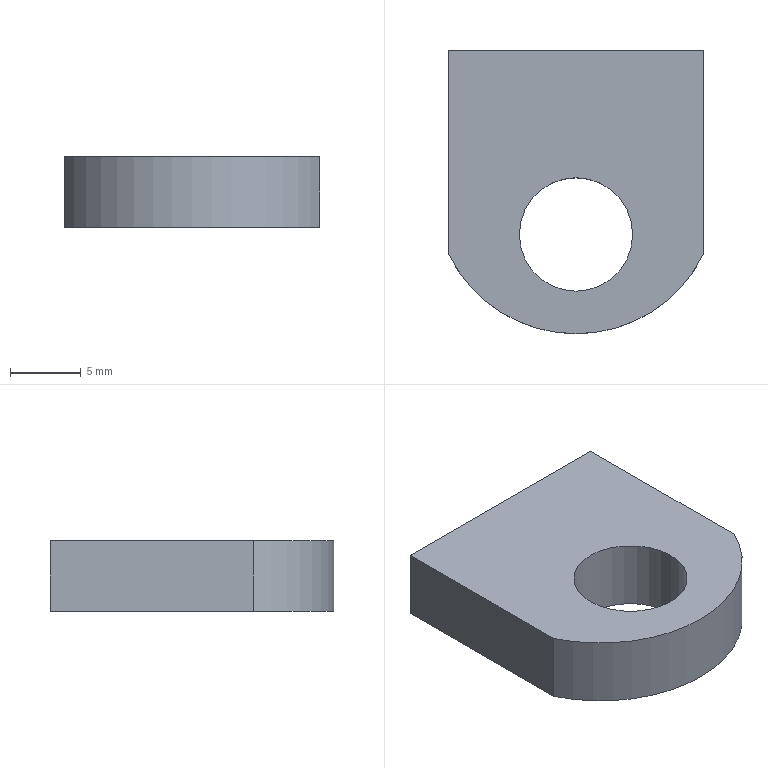Part | SolidWorks | features BaseBody 1 | 1 solid | 14 faces | box 18 x 20 x 5 mm | volume 1306 mm3 | cylinder 7 | plane 7 | commonest cylinder face diameters 3 x4 8 x2 20 x1
STEP:
#1=CARTESIAN_POINT('',(925.946,-4411.473,874.971));
#2=VERTEX_POINT('',#1);
#3=CARTESIAN_POINT('',(917.946,-4411.473,874.971));
#4=VERTEX_POINT('',#3);
#5=CARTESIAN_POINT('',(921.946,-4411.473,874.971));
#6=DIRECTION('',(0.,0.,-1.));
#7=DIRECTION('',(1.,0.,0.));
#8=AXIS2_PLACEMENT_3D('',#5,#6,#7);
#9=CIRCLE('',#8,4.);
#10=EDGE_CURVE('',#2,#4,#9,.T.);
#11=ORIENTED_EDGE('',*,*,#10,.T.);
#12=CARTESIAN_POINT('',(917.946,-4411.473,879.971));
#13=VERTEX_POINT('',#12);
#14=CARTESIAN_POINT('',(917.946,-4411.473,874.971));
#15=DIRECTION('',(0.,0.,1.));
#16=VECTOR('',#15,1000.);
#17=LINE('',#14,#16);
#18=EDGE_CURVE('',#4,#13,#17,.T.);
#19=ORIENTED_EDGE('',*,*,#18,.T.);
#20=CARTESIAN_POINT('',(925.946,-4411.473,879.971));
#21=VERTEX_POINT('',#20);
#22=CARTESIAN_POINT('',(921.946,-4411.473,879.971));
#23=DIRECTION('',(0.,0.,1.));
#24=DIRECTION('',(1.,0.,0.));
#25=AXIS2_PLACEMENT_3D('',#22,#23,#24);
#26=CIRCLE('',#25,4.);
#27=EDGE_CURVE('',#13,#21,#26,.T.);
#28=ORIENTED_EDGE('',*,*,#27,.T.);
#29=CARTESIAN_POINT('',(925.946,-4411.473,874.971));
#30=DIRECTION('',(0.,0.,1.));
#31=VECTOR('',#30,1000.);
#32=LINE('',#29,#31);
#33=EDGE_CURVE('',#2,#21,#32,.T.);
#34=ORIENTED_EDGE('',*,*,#33,.F.);
#35=EDGE_LOOP('',(#11,#19,#28,#34));
#36=FACE_OUTER_BOUND('',#35,.T.);
#37=CARTESIAN_POINT('',(921.946,-4411.473,874.971));
#38=DIRECTION('',(0.,0.,1.));
#39=DIRECTION('',(1.,0.,0.));
#40=AXIS2_PLACEMENT_3D('',#37,#38,#39);
#41=CYLINDRICAL_SURFACE('',#40,4.);
#42=ADVANCED_FACE('',(#36),#41,.F.);
#43=CARTESIAN_POINT('',(916.946,-4398.473,878.971));
#44=VERTEX_POINT('',#43);
#45=CARTESIAN_POINT('',(916.946,-4398.473,875.971));
#46=VERTEX_POINT('',#45);
#47=CARTESIAN_POINT('',(916.946,-4398.473,877.471));
#48=DIRECTION('',(0.,-1.,0.));
#49=DIRECTION('',(0.,0.,-1.));
#50=AXIS2_PLACEMENT_3D('',#47,#48,#49);
#51=CIRCLE('',#50,1.5);
#52=EDGE_CURVE('',#44,#46,#51,.T.);
#53=ORIENTED_EDGE('',*,*,#52,.F.);
#54=CARTESIAN_POINT('',(916.946,-4405.473,878.971));
#55=VERTEX_POINT('',#54);
#56=CARTESIAN_POINT('',(916.946,-4385.473,878.971));
#57=DIRECTION('',(0.,-1.,0.));
#58=VECTOR('',#57,1000.);
#59=LINE('',#56,#58);
#60=EDGE_CURVE('',#44,#55,#59,.T.);
#61=ORIENTED_EDGE('',*,*,#60,.T.);
#62=CARTESIAN_POINT('',(916.946,-4405.473,875.971));
#63=VERTEX_POINT('',#62);
#64=CARTESIAN_POINT('',(916.946,-4405.473,877.471));
#65=DIRECTION('',(0.,1.,0.));
#66=DIRECTION('',(0.,0.,-1.));
#67=AXIS2_PLACEMENT_3D('',#64,#65,#66);
#68=CIRCLE('',#67,1.5);
#69=EDGE_CURVE('',#63,#55,#68,.T.);
#70=ORIENTED_EDGE('',*,*,#69,.F.);
#71=CARTESIAN_POINT('',(916.946,-4385.473,875.971));
#72=DIRECTION('',(0.,-1.,0.));
#73=VECTOR('',#72,1000.);
#74=LINE('',#71,#73);
#75=EDGE_CURVE('',#46,#63,#74,.T.);
#76=ORIENTED_EDGE('',*,*,#75,.F.);
#77=EDGE_LOOP('',(#53,#61,#70,#76));
#78=FACE_OUTER_BOUND('',#77,.T.);
#79=CARTESIAN_POINT('',(916.946,-4385.473,877.471));
#80=DIRECTION('',(0.,-1.,0.));
#81=DIRECTION('',(0.,0.,-1.));
#82=AXIS2_PLACEMENT_3D('',#79,#80,#81);
#83=CYLINDRICAL_SURFACE('',#82,1.5);
#84=ADVANCED_FACE('',(#78),#83,.F.);
#85=CARTESIAN_POINT('',(926.978,-4405.473,875.971));
#86=VERTEX_POINT('',#85);
#87=CARTESIAN_POINT('',(926.978,-4405.473,878.971));
#88=VERTEX_POINT('',#87);
#89=CARTESIAN_POINT('',(926.978,-4405.473,877.471));
#90=DIRECTION('',(0.,1.,0.));
#91=DIRECTION('',(0.,0.,1.));
#92=AXIS2_PLACEMENT_3D('',#89,#90,#91);
#93=CIRCLE('',#92,1.5);
#94=EDGE_CURVE('',#86,#88,#93,.T.);
#95=ORIENTED_EDGE('',*,*,#94,.F.);
#96=CARTESIAN_POINT('',(926.978,-4398.473,875.971));
#97=VERTEX_POINT('',#96);
#98=CARTESIAN_POINT('',(926.978,-4385.473,875.971));
#99=DIRECTION('',(0.,1.,0.));
#100=VECTOR('',#99,1000.);
#101=LINE('',#98,#100);
#102=EDGE_CURVE('',#86,#97,#101,.T.);
#103=ORIENTED_EDGE('',*,*,#102,.T.);
#104=CARTESIAN_POINT('',(926.978,-4398.473,878.971));
#105=VERTEX_POINT('',#104);
#106=CARTESIAN_POINT('',(926.978,-4398.473,877.471));
#107=DIRECTION('',(0.,-1.,0.));
#108=DIRECTION('',(0.,0.,1.));
#109=AXIS2_PLACEMENT_3D('',#106,#107,#108);
#110=CIRCLE('',#109,1.5);
#111=EDGE_CURVE('',#105,#97,#110,.T.);
#112=ORIENTED_EDGE('',*,*,#111,.F.);
#113=CARTESIAN_POINT('',(926.978,-4385.473,878.971));
#114=DIRECTION('',(0.,1.,0.));
#115=VECTOR('',#114,1000.);
#116=LINE('',#113,#115);
#117=EDGE_CURVE('',#88,#105,#116,.T.);
#118=ORIENTED_EDGE('',*,*,#117,.F.);
#119=EDGE_LOOP('',(#95,#103,#112,#118));
#120=FACE_OUTER_BOUND('',#119,.T.);
#121=CARTESIAN_POINT('',(926.978,-4385.473,877.471));
#122=DIRECTION('',(0.,1.,0.));
#123=DIRECTION('',(0.,0.,1.));
#124=AXIS2_PLACEMENT_3D('',#121,#122,#123);
#125=CYLINDRICAL_SURFACE('',#124,1.5);
#126=ADVANCED_FACE('',(#120),#125,.F.);
#127=CARTESIAN_POINT('',(930.946,-4398.473,874.971));
#128=VERTEX_POINT('',#127);
#129=CARTESIAN_POINT('',(912.946,-4398.473,874.971));
#130=VERTEX_POINT('',#129);
#131=CARTESIAN_POINT('',(921.946,-4398.473,874.971));
#132=DIRECTION('',(-1.,0.,0.));
#133=VECTOR('',#132,1000.);
#134=LINE('',#131,#133);
#135=EDGE_CURVE('',#128,#130,#134,.T.);
#136=ORIENTED_EDGE('',*,*,#135,.F.);
#137=CARTESIAN_POINT('',(930.946,-4412.832,874.971));
#138=VERTEX_POINT('',#137);
#139=CARTESIAN_POINT('',(930.946,-4406.797,874.971));
#140=DIRECTION('',(0.,1.,0.));
#141=VECTOR('',#140,1000.);
#142=LINE('',#139,#141);
#143=EDGE_CURVE('',#138,#128,#142,.T.);
#144=ORIENTED_EDGE('',*,*,#143,.F.);
#145=CARTESIAN_POINT('',(912.946,-4412.832,874.971));
#146=VERTEX_POINT('',#145);
#147=CARTESIAN_POINT('',(921.946,-4408.473,874.971));
#148=DIRECTION('',(0.,0.,1.));
#149=DIRECTION('',(1.,0.,0.));
#150=AXIS2_PLACEMENT_3D('',#147,#148,#149);
#151=CIRCLE('',#150,10.);
#152=EDGE_CURVE('',#146,#138,#151,.T.);
#153=ORIENTED_EDGE('',*,*,#152,.F.);
#154=CARTESIAN_POINT('',(912.946,-4406.797,874.971));
#155=DIRECTION('',(0.,-1.,0.));
#156=VECTOR('',#155,1000.);
#157=LINE('',#154,#156);
#158=EDGE_CURVE('',#130,#146,#157,.T.);
#159=ORIENTED_EDGE('',*,*,#158,.F.);
#160=EDGE_LOOP('',(#136,#144,#153,#159));
#161=FACE_OUTER_BOUND('',#160,.T.);
#162=ORIENTED_EDGE('',*,*,#10,.F.);
#163=CARTESIAN_POINT('',(921.946,-4411.473,874.971));
#164=DIRECTION('',(0.,0.,-1.));
#165=DIRECTION('',(1.,0.,0.));
#166=AXIS2_PLACEMENT_3D('',#163,#164,#165);
#167=CIRCLE('',#166,4.);
#168=EDGE_CURVE('',#4,#2,#167,.T.);
#169=ORIENTED_EDGE('',*,*,#168,.F.);
#170=EDGE_LOOP('',(#162,#169));
#171=FACE_BOUND('',#170,.T.);
#172=CARTESIAN_POINT('',(921.946,-4406.797,874.971));
#173=DIRECTION('',(0.,0.,1.));
#174=DIRECTION('',(1.,0.,0.));
#175=AXIS2_PLACEMENT_3D('',#172,#173,#174);
#176=PLANE('',#175);
#177=ADVANCED_FACE('',(#161,#171),#176,.F.);
#178=ORIENTED_EDGE('',*,*,#158,.T.);
#179=CARTESIAN_POINT('',(912.946,-4412.832,879.971));
#180=VERTEX_POINT('',#179);
#181=CARTESIAN_POINT('',(912.946,-4412.832,874.971));
#182=DIRECTION('',(0.,0.,1.));
#183=VECTOR('',#182,1000.);
#184=LINE('',#181,#183);
#185=EDGE_CURVE('',#146,#180,#184,.T.);
#186=ORIENTED_EDGE('',*,*,#185,.T.);
#187=CARTESIAN_POINT('',(912.946,-4398.473,879.971));
#188=VERTEX_POINT('',#187);
#189=CARTESIAN_POINT('',(912.946,-4408.473,879.971));
#190=DIRECTION('',(0.,1.,0.));
#191=VECTOR('',#190,1000.);
#192=LINE('',#189,#191);
#193=EDGE_CURVE('',#180,#188,#192,.T.);
#194=ORIENTED_EDGE('',*,*,#193,.T.);
#195=CARTESIAN_POINT('',(912.946,-4398.473,874.971));
#196=DIRECTION('',(0.,0.,-1.));
#197=VECTOR('',#196,1000.);
#198=LINE('',#195,#197);
#199=EDGE_CURVE('',#188,#130,#198,.T.);
#200=ORIENTED_EDGE('',*,*,#199,.T.);
#201=EDGE_LOOP('',(#178,#186,#194,#200));
#202=FACE_OUTER_BOUND('',#201,.T.);
#203=CARTESIAN_POINT('',(912.946,-4408.473,874.971));
#204=DIRECTION('',(-1.,0.,0.));
#205=DIRECTION('',(0.,0.,1.));
#206=AXIS2_PLACEMENT_3D('',#203,#204,#205);
#207=PLANE('',#206);
#208=ADVANCED_FACE('',(#202),#207,.T.);
#209=ORIENTED_EDGE('',*,*,#135,.T.);
#210=ORIENTED_EDGE('',*,*,#199,.F.);
#211=CARTESIAN_POINT('',(930.946,-4398.473,879.971));
#212=VERTEX_POINT('',#211);
#213=CARTESIAN_POINT('',(911.946,-4398.473,879.971));
#214=DIRECTION('',(1.,0.,0.));
#215=VECTOR('',#214,1000.);
#216=LINE('',#213,#215);
#217=EDGE_CURVE('',#188,#212,#216,.T.);
#218=ORIENTED_EDGE('',*,*,#217,.T.);
#219=CARTESIAN_POINT('',(930.946,-4398.473,874.971));
#220=DIRECTION('',(0.,0.,-1.));
#221=VECTOR('',#220,1000.);
#222=LINE('',#219,#221);
#223=EDGE_CURVE('',#212,#128,#222,.T.);
#224=ORIENTED_EDGE('',*,*,#223,.T.);
#225=EDGE_LOOP('',(#209,#210,#218,#224));
#226=FACE_OUTER_BOUND('',#225,.T.);
#227=CARTESIAN_POINT('',(916.946,-4398.473,877.471));
#228=DIRECTION('',(0.,-1.,0.));
#229=DIRECTION('',(0.,0.,-1.));
#230=AXIS2_PLACEMENT_3D('',#227,#228,#229);
#231=CIRCLE('',#230,1.5);
#232=EDGE_CURVE('',#46,#44,#231,.T.);
#233=ORIENTED_EDGE('',*,*,#232,.T.);
#234=ORIENTED_EDGE('',*,*,#52,.T.);
#235=EDGE_LOOP('',(#233,#234));
#236=FACE_BOUND('',#235,.T.);
#237=ORIENTED_EDGE('',*,*,#111,.T.);
#238=CARTESIAN_POINT('',(926.978,-4398.473,877.471));
#239=DIRECTION('',(0.,-1.,0.));
#240=DIRECTION('',(0.,0.,1.));
#241=AXIS2_PLACEMENT_3D('',#238,#239,#240);
#242=CIRCLE('',#241,1.5);
#243=EDGE_CURVE('',#97,#105,#242,.T.);
#244=ORIENTED_EDGE('',*,*,#243,.T.);
#245=EDGE_LOOP('',(#237,#244));
#246=FACE_BOUND('',#245,.T.);
#247=CARTESIAN_POINT('',(911.946,-4398.473,874.971));
#248=DIRECTION('',(0.,1.,0.));
#249=DIRECTION('',(0.,0.,1.));
#250=AXIS2_PLACEMENT_3D('',#247,#248,#249);
#251=PLANE('',#250);
#252=ADVANCED_FACE('',(#226,#236,#246),#251,.T.);
#253=ORIENTED_EDGE('',*,*,#143,.T.);
#254=ORIENTED_EDGE('',*,*,#223,.F.);
#255=CARTESIAN_POINT('',(930.946,-4412.832,879.971));
#256=VERTEX_POINT('',#255);
#257=CARTESIAN_POINT('',(930.946,-4398.473,879.971));
#258=DIRECTION('',(0.,-1.,0.));
#259=VECTOR('',#258,1000.);
#260=LINE('',#257,#259);
#261=EDGE_CURVE('',#212,#256,#260,.T.);
#262=ORIENTED_EDGE('',*,*,#261,.T.);
#263=CARTESIAN_POINT('',(930.946,-4412.832,874.971));
#264=DIRECTION('',(0.,0.,-1.));
#265=VECTOR('',#264,1000.);
#266=LINE('',#263,#265);
#267=EDGE_CURVE('',#256,#138,#266,.T.);
#268=ORIENTED_EDGE('',*,*,#267,.T.);
#269=EDGE_LOOP('',(#253,#254,#262,#268));
#270=FACE_OUTER_BOUND('',#269,.T.);
#271=CARTESIAN_POINT('',(930.946,-4398.473,874.971));
#272=DIRECTION('',(1.,0.,0.));
#273=DIRECTION('',(0.,0.,-1.));
#274=AXIS2_PLACEMENT_3D('',#271,#272,#273);
#275=PLANE('',#274);
#276=ADVANCED_FACE('',(#270),#275,.T.);
#277=ORIENTED_EDGE('',*,*,#152,.T.);
#278=ORIENTED_EDGE('',*,*,#267,.F.);
#279=CARTESIAN_POINT('',(921.946,-4408.473,879.971));
#280=DIRECTION('',(0.,0.,-1.));
#281=DIRECTION('',(1.,0.,0.));
#282=AXIS2_PLACEMENT_3D('',#279,#280,#281);
#283=CIRCLE('',#282,10.);
#284=EDGE_CURVE('',#256,#180,#283,.T.);
#285=ORIENTED_EDGE('',*,*,#284,.T.);
#286=ORIENTED_EDGE('',*,*,#185,.F.);
#287=EDGE_LOOP('',(#277,#278,#285,#286));
#288=FACE_OUTER_BOUND('',#287,.T.);
#289=CARTESIAN_POINT('',(921.946,-4408.473,874.971));
#290=DIRECTION('',(0.,0.,1.));
#291=DIRECTION('',(1.,0.,0.));
#292=AXIS2_PLACEMENT_3D('',#289,#290,#291);
#293=CYLINDRICAL_SURFACE('',#292,10.);
#294=ADVANCED_FACE('',(#288),#293,.T.);
#295=ORIENTED_EDGE('',*,*,#18,.F.);
#296=ORIENTED_EDGE('',*,*,#168,.T.);
#297=ORIENTED_EDGE('',*,*,#33,.T.);
#298=CARTESIAN_POINT('',(921.946,-4411.473,879.971));
#299=DIRECTION('',(0.,0.,1.));
#300=DIRECTION('',(1.,0.,0.));
#301=AXIS2_PLACEMENT_3D('',#298,#299,#300);
#302=CIRCLE('',#301,4.);
#303=EDGE_CURVE('',#21,#13,#302,.T.);
#304=ORIENTED_EDGE('',*,*,#303,.T.);
#305=EDGE_LOOP('',(#295,#296,#297,#304));
#306=FACE_OUTER_BOUND('',#305,.T.);
#307=CARTESIAN_POINT('',(921.946,-4411.473,874.971));
#308=DIRECTION('',(0.,0.,1.));
#309=DIRECTION('',(1.,0.,0.));
#310=AXIS2_PLACEMENT_3D('',#307,#308,#309);
#311=CYLINDRICAL_SURFACE('',#310,4.);
#312=ADVANCED_FACE('',(#306),#311,.F.);
#313=ORIENTED_EDGE('',*,*,#284,.F.);
#314=ORIENTED_EDGE('',*,*,#261,.F.);
#315=ORIENTED_EDGE('',*,*,#217,.F.);
#316=ORIENTED_EDGE('',*,*,#193,.F.);
#317=EDGE_LOOP('',(#313,#314,#315,#316));
#318=FACE_OUTER_BOUND('',#317,.T.);
#319=ORIENTED_EDGE('',*,*,#303,.F.);
#320=ORIENTED_EDGE('',*,*,#27,.F.);
#321=EDGE_LOOP('',(#319,#320));
#322=FACE_BOUND('',#321,.T.);
#323=CARTESIAN_POINT('',(921.946,-4406.797,879.971));
#324=DIRECTION('',(0.,0.,1.));
#325=DIRECTION('',(1.,0.,0.));
#326=AXIS2_PLACEMENT_3D('',#323,#324,#325);
#327=PLANE('',#326);
#328=ADVANCED_FACE('',(#318,#322),#327,.T.);
#329=ORIENTED_EDGE('',*,*,#60,.F.);
#330=ORIENTED_EDGE('',*,*,#232,.F.);
#331=ORIENTED_EDGE('',*,*,#75,.T.);
#332=CARTESIAN_POINT('',(916.946,-4405.473,877.471));
#333=DIRECTION('',(0.,1.,0.));
#334=DIRECTION('',(0.,0.,-1.));
#335=AXIS2_PLACEMENT_3D('',#332,#333,#334);
#336=CIRCLE('',#335,1.5);
#337=EDGE_CURVE('',#55,#63,#336,.T.);
#338=ORIENTED_EDGE('',*,*,#337,.F.);
#339=EDGE_LOOP('',(#329,#330,#331,#338));
#340=FACE_OUTER_BOUND('',#339,.T.);
#341=CARTESIAN_POINT('',(916.946,-4385.473,877.471));
#342=DIRECTION('',(0.,-1.,0.));
#343=DIRECTION('',(0.,0.,-1.));
#344=AXIS2_PLACEMENT_3D('',#341,#342,#343);
#345=CYLINDRICAL_SURFACE('',#344,1.5);
#346=ADVANCED_FACE('',(#340),#345,.F.);
#347=ORIENTED_EDGE('',*,*,#102,.F.);
#348=CARTESIAN_POINT('',(926.978,-4405.473,877.471));
#349=DIRECTION('',(0.,1.,0.));
#350=DIRECTION('',(0.,0.,1.));
#351=AXIS2_PLACEMENT_3D('',#348,#349,#350);
#352=CIRCLE('',#351,1.5);
#353=EDGE_CURVE('',#88,#86,#352,.T.);
#354=ORIENTED_EDGE('',*,*,#353,.F.);
#355=ORIENTED_EDGE('',*,*,#117,.T.);
#356=ORIENTED_EDGE('',*,*,#243,.F.);
#357=EDGE_LOOP('',(#347,#354,#355,#356));
#358=FACE_OUTER_BOUND('',#357,.T.);
#359=CARTESIAN_POINT('',(926.978,-4385.473,877.471));
#360=DIRECTION('',(0.,1.,0.));
#361=DIRECTION('',(0.,0.,1.));
#362=AXIS2_PLACEMENT_3D('',#359,#360,#361);
#363=CYLINDRICAL_SURFACE('',#362,1.5);
#364=ADVANCED_FACE('',(#358),#363,.F.);
#365=ORIENTED_EDGE('',*,*,#69,.T.);
#366=ORIENTED_EDGE('',*,*,#337,.T.);
#367=EDGE_LOOP('',(#365,#366));
#368=FACE_OUTER_BOUND('',#367,.T.);
#369=CARTESIAN_POINT('',(916.946,-4405.473,877.471));
#370=DIRECTION('',(0.,-1.,0.));
#371=DIRECTION('',(0.,0.,-1.));
#372=AXIS2_PLACEMENT_3D('',#369,#370,#371);
#373=PLANE('',#372);
#374=ADVANCED_FACE('',(#368),#373,.F.);
#375=ORIENTED_EDGE('',*,*,#353,.T.);
#376=ORIENTED_EDGE('',*,*,#94,.T.);
#377=EDGE_LOOP('',(#375,#376));
#378=FACE_OUTER_BOUND('',#377,.T.);
#379=CARTESIAN_POINT('',(926.978,-4405.473,877.471));
#380=DIRECTION('',(0.,-1.,0.));
#381=DIRECTION('',(0.,0.,-1.));
#382=AXIS2_PLACEMENT_3D('',#379,#380,#381);
#383=PLANE('',#382);
#384=ADVANCED_FACE('',(#378),#383,.F.);
#385=CLOSED_SHELL('',(#42,#84,#126,#177,#208,#252,#276,#294,#312,#328,#346,#364,#374,#384));
#386=MANIFOLD_SOLID_BREP('',#385);
#387=CARTESIAN_POINT('',(0.,0.,0.));
#388=DIRECTION('',(0.,0.,1.));
#389=DIRECTION('',(1.,0.,0.));
#390=AXIS2_PLACEMENT_3D('',#387,#388,#389);
#391=(LENGTH_UNIT()NAMED_UNIT(*)SI_UNIT(.MILLI.,.METRE.));
#392=UNCERTAINTY_MEASURE_WITH_UNIT(LENGTH_MEASURE(0.00001),#391,'','');
#393=(NAMED_UNIT(*)PLANE_ANGLE_UNIT()SI_UNIT($,.RADIAN.));
#394=(NAMED_UNIT(*)SI_UNIT($,.STERADIAN.)SOLID_ANGLE_UNIT());
#395=(GEOMETRIC_REPRESENTATION_CONTEXT(3)GLOBAL_UNCERTAINTY_ASSIGNED_CONTEXT((#392))GLOBAL_UNIT_ASSIGNED_CONTEXT((#391,#393,#394))REPRESENTATION_CONTEXT('',''));
#396=ADVANCED_BREP_SHAPE_REPRESENTATION('',(#386,#390),#395);